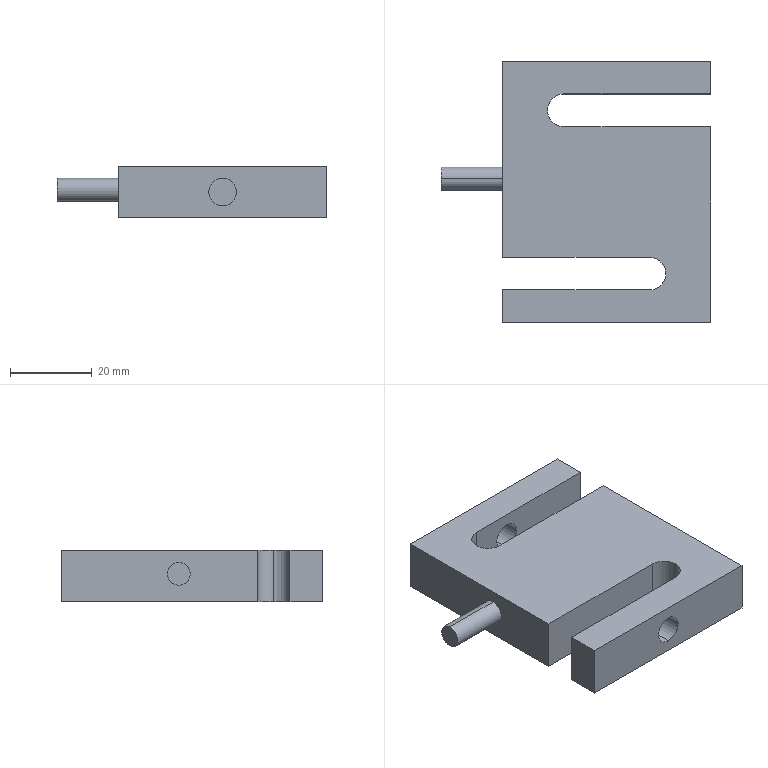Part | STEP file | ASND-0110-YD02 | 1 solid | 22 faces | box 66 x 64 x 12.7 mm | volume 33292 mm3 | plane 13 | cylinder 9 | commonest cylinder face diameters 6.8 x4 8 x3 5.637 x2